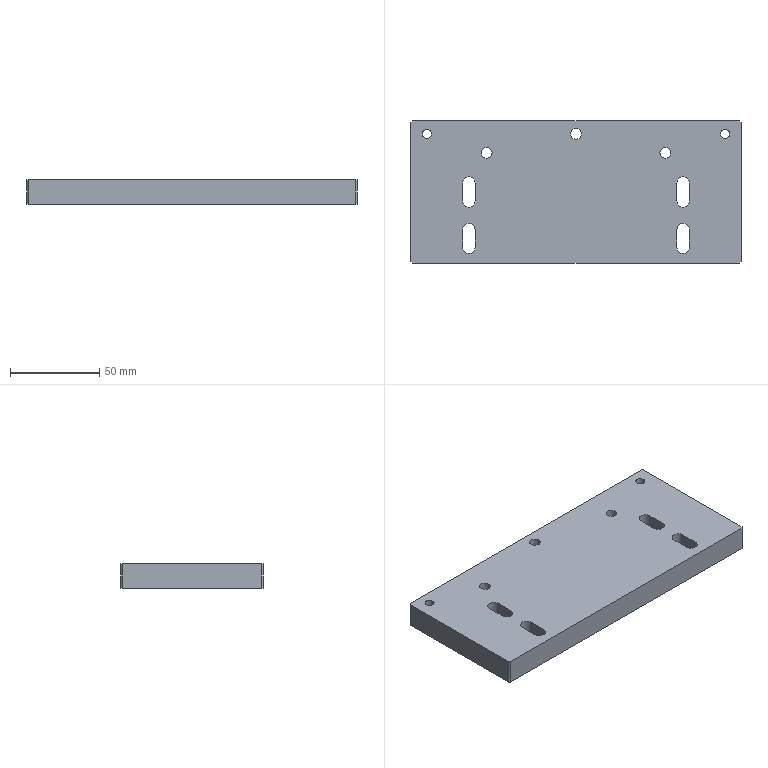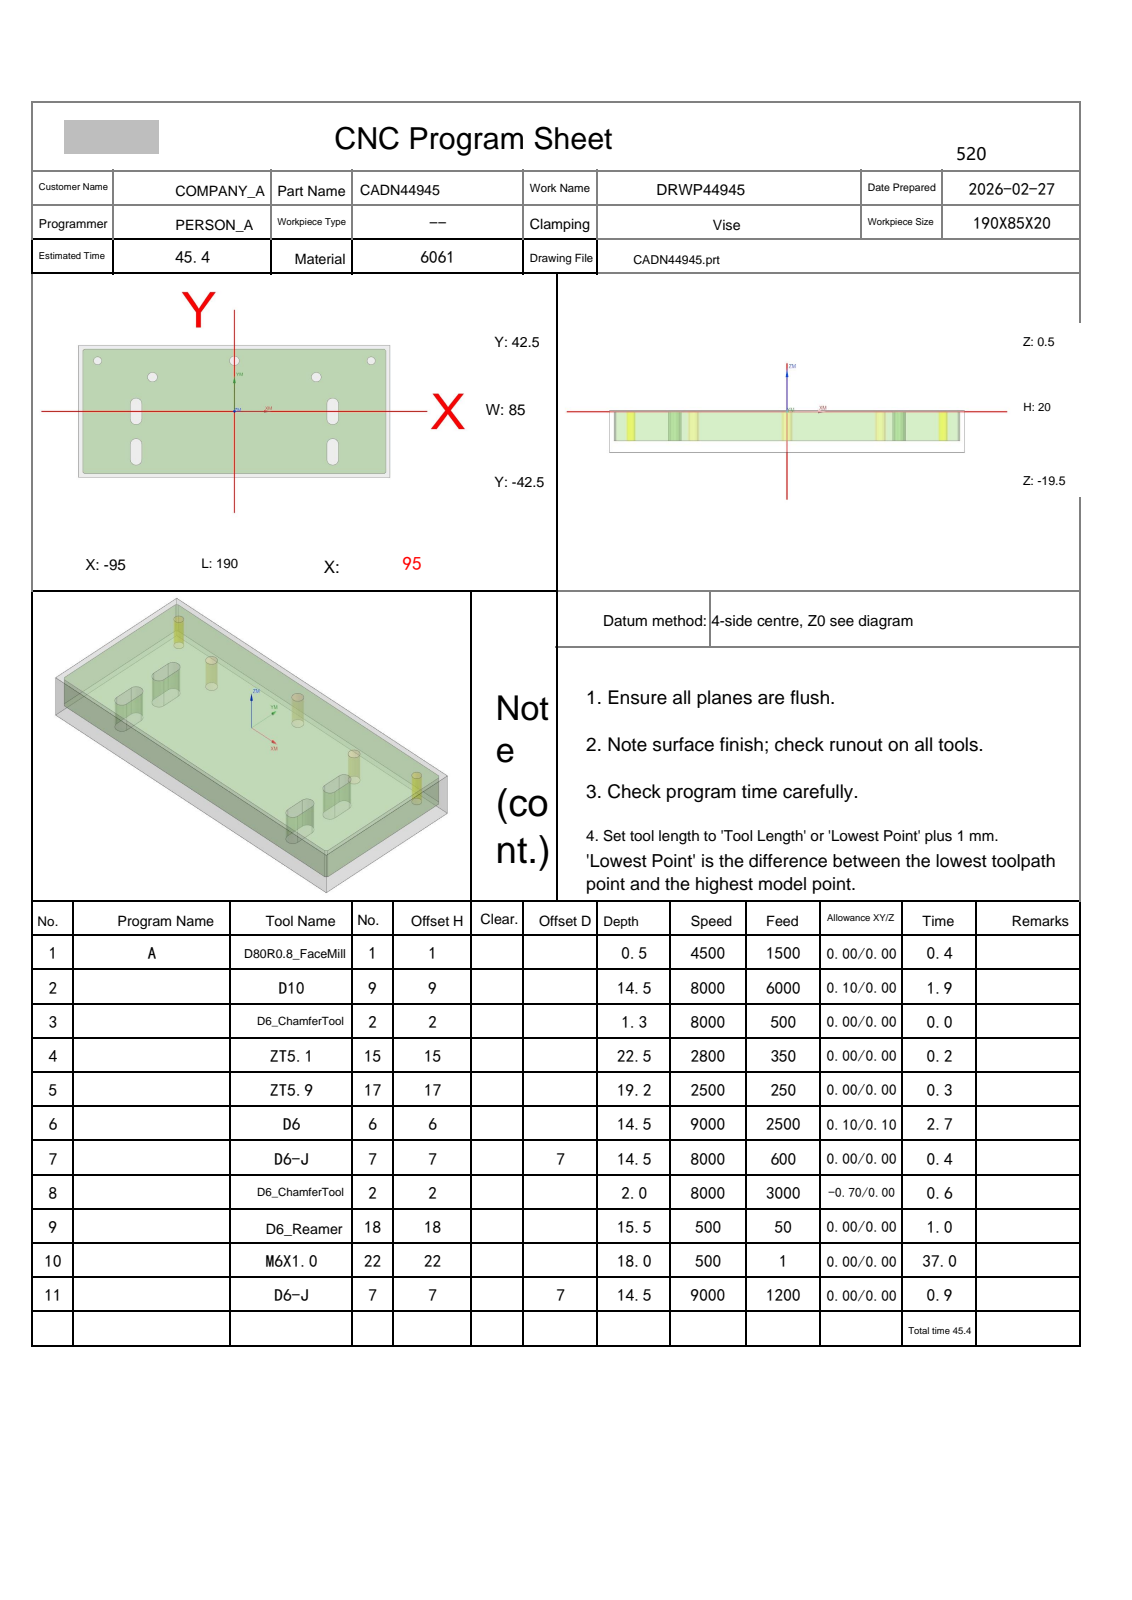NC program | NX | posted by the shop | part box 185 x 80 x 14 mm
Lines 2325 to 2772 of 2772:
N7 T07 M06
(D6-J  D=6. R=0. H=07 ce=0.00 di=0.00)
G00 G90 G54 X-59.75 Y-26.2 M03 S8000
G43 H07 Z50.
M08
Z-6.5
G01 Z-7. F600.
G41 D07
X-59.7
G03 X-59.5 Y-26. I0.0 J.2
G01 Y-21.
G03 X-60. Y-20.5 I-.5 J0.0
X-60.5 Y-21. I0.0 J-.5
G01 Y-31.
G03 X-60. Y-31.5 I.5 J0.0
X-59.5 Y-31. I0.0 J.5
G01 Y-26.
Y-25.5
G03 X-59.7 Y-25.3 I-.2 J0.0
G01 G40 X-59.75
Z-6.5
G00 Z1.
Y-26.2
Z-13.5
G01 Z-14.
G41 D07
X-59.7
G03 X-59.5 Y-26. I0.0 J.2
G01 Y-21.
G03 X-60. Y-20.5 I-.5 J0.0
X-60.5 Y-21. I0.0 J-.5
G01 Y-31.
G03 X-60. Y-31.5 I.5 J0.0
X-59.5 Y-31. I0.0 J.5
G01 Y-26.
Y-25.5
G03 X-59.7 Y-25.3 I-.2 J0.0
G01 G40 X-59.75
Z-13.5
G00 Z50.
Y-.2
Z-6.5
G01 Z-7.
G41 D07
X-59.7
G03 X-59.5 Y0.0 I0.0 J.2
G01 Y5.
G03 X-60. Y5.5 I-.5 J0.0
X-60.5 Y5. I0.0 J-.5
G01 Y-5.
G03 X-60. Y-5.5 I.5 J0.0
X-59.5 Y-5. I0.0 J.5
G01 Y0.0
Y.5
G03 X-59.7 Y.7 I-.2 J0.0
G01 G40 X-59.75
Z-6.5
G00 Z1.
Y-.2
Z-13.5
G01 Z-14.
G41 D07
X-59.7
G03 X-59.5 Y0.0 I0.0 J.2
G01 Y5.
G03 X-60. Y5.5 I-.5 J0.0
X-60.5 Y5. I0.0 J-.5
G01 Y-5.
G03 X-60. Y-5.5 I.5 J0.0
X-59.5 Y-5. I0.0 J.5
G01 Y0.0
Y.5
G03 X-59.7 Y.7 I-.2 J0.0
G01 G40 X-59.75
Z-13.5
G00 Z50.
X60.25 Y-26.2
Z-6.5
G01 Z-7.
G41 D07
X60.3
G03 X60.5 Y-26. I0.0 J.2
G01 Y-21.
G03 X60. Y-20.5 I-.5 J0.0
X59.5 Y-21. I0.0 J-.5
G01 Y-31.
G03 X60. Y-31.5 I.5 J0.0
X60.5 Y-31. I0.0 J.5
G01 Y-26.
Y-25.5
G03 X60.3 Y-25.3 I-.2 J0.0
G01 G40 X60.25
Z-6.5
G00 Z1.
Y-26.2
Z-13.5
G01 Z-14.
G41 D07
X60.3
G03 X60.5 Y-26. I0.0 J.2
G01 Y-21.
G03 X60. Y-20.5 I-.5 J0.0
X59.5 Y-21. I0.0 J-.5
G01 Y-31.
G03 X60. Y-31.5 I.5 J0.0
X60.5 Y-31. I0.0 J.5
G01 Y-26.
Y-25.5
G03 X60.3 Y-25.3 I-.2 J0.0
G01 G40 X60.25
Z-13.5
G00 Z50.
Y-.2
Z-6.5
G01 Z-7.
G41 D07
X60.3
G03 X60.5 Y0.0 I0.0 J.2
G01 Y5.
G03 X60. Y5.5 I-.5 J0.0
X59.5 Y5. I0.0 J-.5
G01 Y-5.
G03 X60. Y-5.5 I.5 J0.0
X60.5 Y-5. I0.0 J.5
G01 Y0.0
Y.5
G03 X60.3 Y.7 I-.2 J0.0
G01 G40 X60.25
Z-6.5
G00 Z1.
Y-.2
Z-13.5
G01 Z-14.
G41 D07
X60.3
G03 X60.5 Y0.0 I0.0 J.2
G01 Y5.
G03 X60. Y5.5 I-.5 J0.0
X59.5 Y5. I0.0 J-.5
G01 Y-5.
G03 X60. Y-5.5 I.5 J0.0
X60.5 Y-5. I0.0 J.5
G01 Y0.0
Y.5
G03 X60.3 Y.7 I-.2 J0.0
G01 G40 X60.25
Z-13.5
G00 Z50.
G91 G28 Z0.0
M05
M09
G91 G28 Z0.0
M01
N8 T02 M06
(D6_ChamferTool  D=6. R=0. H=02 ce=0.00 di=0.00)
G00 G90 G54 X-.25 Y42.128 M03 S8000
G43 H02 Z50.
M08
Z2.099
G01 Z-1.5 F3000.
G03 X-.33 Y41.828 I.52 J-.3
X-.03 Y41.308 I.6 J0.0
G01 X0.0 Y41.3
X91.5
X91.754 Y41.275
X91.997 Y41.201
X92.222 Y41.081
X92.419 Y40.919
X93.419 Y39.919
X93.581 Y39.722
X93.701 Y39.497
X93.775 Y39.254
X93.8 Y39.
Y-39.
X93.775 Y-39.254
X93.701 Y-39.497
X93.581 Y-39.722
X93.419 Y-39.919
X92.419 Y-40.919
X92.222 Y-41.081
X91.997 Y-41.201
X91.754 Y-41.275
X91.5 Y-41.3
X-91.5
X-91.753 Y-41.275
X-91.997 Y-41.201
X-92.222 Y-41.081
X-92.419 Y-40.919
X-93.419 Y-39.919
X-93.581 Y-39.722
X-93.701 Y-39.497
X-93.775 Y-39.254
X-93.8 Y-39.
Y39.
X-93.775 Y39.254
X-93.701 Y39.497
X-93.581 Y39.722
X-93.419 Y39.919
X-92.419 Y40.919
X-92.222 Y41.081
X-91.997 Y41.201
X-91.754 Y41.275
X-91.5 Y41.3
X0.0
X.03 Y41.308
G03 X.33 Y41.828 I-.3 J.52
X.25 Y42.128 I-.6 J0.0
G01 Z2.099
G00 Z50.
X58.628 Y-25.75
Z2.099
G01 Z-1.5
G03 X58.328 Y-25.67 I-.3 J-.52
X57.808 Y-25.97 I0.0 J-.6
G01 X57.8 Y-26.
Y-31.
G03 X60. Y-33.2 I2.2 J0.0
X62.2 Y-31. I0.0 J2.2
G01 Y-21.
G03 X60. Y-18.8 I-2.2 J0.0
X57.8 Y-21. I0.0 J-2.2
G01 Y-26.
X57.808 Y-26.03
G03 X58.328 Y-26.33 I.52 J.3
X58.628 Y-26.25 I0.0 J.6
G01 Z2.099
G00 Z50.
Y.25
Z2.099
G01 Z-1.5
G03 X58.328 Y.33 I-.3 J-.52
X57.808 Y.03 I0.0 J-.6
G01 X57.8 Y0.0
Y-5.
G03 X60. Y-7.2 I2.2 J0.0
X62.2 Y-5. I0.0 J2.2
G01 Y5.
G03 X60. Y7.2 I-2.2 J0.0
X57.8 Y5. I0.0 J-2.2
G01 Y0.0
X57.808 Y-.03
G03 X58.328 Y-.33 I.52 J.3
X58.628 Y-.25 I0.0 J.6
G01 Z2.099
G00 Z50.
X-58.628
Z2.099
G01 Z-1.5
G03 X-58.328 Y-.33 I.3 J.52
X-57.808 Y-.03 I0.0 J.6
G01 X-57.8 Y0.0
Y5.
G03 X-60. Y7.2 I-2.2 J0.0
X-62.2 Y5. I0.0 J-2.2
G01 Y-5.
G03 X-60. Y-7.2 I2.2 J0.0
X-57.8 Y-5. I0.0 J2.2
G01 Y0.0
X-57.808 Y.03
G03 X-58.328 Y.33 I-.52 J-.3
X-58.628 Y.25 I0.0 J-.6
G01 Z2.099
G00 Z50.
Y-26.25
Z2.099
G01 Z-1.5
G03 X-58.328 Y-26.33 I.3 J.52
X-57.808 Y-26.03 I0.0 J.6
G01 X-57.8 Y-26.
Y-21.
G03 X-60. Y-18.8 I-2.2 J0.0
X-62.2 Y-21. I0.0 J-2.2
G01 Y-31.
G03 X-60. Y-33.2 I2.2 J0.0
X-57.8 Y-31. I0.0 J2.2
G01 Y-26.
X-57.808 Y-25.97
G03 X-58.328 Y-25.67 I-.52 J-.3
X-58.628 Y-25.75 I0.0 J-.6
G01 Z2.099
G00 Z50.
G00 G90 X-83.909 Y33.521 M03 S8000
Z50.
Z-.6
G01 Z-1.1 F500.
X-84.1 Y34.
G03 X-85.6 Y32.5 I0.0 J-1.5
X-83.5 Y30.4 I2.1 J0.0
X-81.4 Y32.5 I0.0 J2.1
X-83.5 Y34.6 I-2.1 J0.0
X-85.6 Y32.5 I0.0 J-2.1
X-84.1 Y31. I1.5 J0.0
G01 X-83.909 Y31.479
Z-.6
G00 Z50.
X83.091 Y33.521
Z-.6
G01 Z-1.1
X82.9 Y34.
G03 X81.4 Y32.5 I0.0 J-1.5
X83.5 Y30.4 I2.1 J0.0
X85.6 Y32.5 I0.0 J2.1
X83.5 Y34.6 I-2.1 J0.0
X81.4 Y32.5 I0.0 J-2.1
X82.9 Y31. I1.5 J0.0
G01 X83.091 Y31.479
Z-.6
G00 Z50.
G00 G90 X-50.612 Y23.147 M03 S8000
Z50.
Z-.5
G01 Z-1. F500.
X-50.8 Y23.5
G03 X-52.3 Y22. I0.0 J-1.5
X-50. Y19.7 I2.3 J0.0
X-47.7 Y22. I0.0 J2.3
X-50. Y24.3 I-2.3 J0.0
X-52.3 Y22. I0.0 J-2.3
X-50.8 Y20.5 I1.5 J0.0
G01 X-50.612 Y20.853
Z-.5
G00 Z50.
X-.612 Y33.647
Z-.5
G01 Z-1.
X-.8 Y34.
G03 X-2.3 Y32.5 I0.0 J-1.5
X0.0 Y30.2 I2.3 J0.0
X2.3 Y32.5 I0.0 J2.3
X0.0 Y34.8 I-2.3 J0.0
X-2.3 Y32.5 I0.0 J-2.3
X-.8 Y31. I1.5 J0.0
G01 X-.612 Y31.353
Z-.5
G00 Z50.
X49.388 Y23.147
Z-.5
G01 Z-1.
X49.2 Y23.5
G03 X47.7 Y22. I0.0 J-1.5
X50. Y19.7 I2.3 J0.0
X52.3 Y22. I0.0 J2.3
X50. Y24.3 I-2.3 J0.0
X47.7 Y22. I0.0 J-2.3
X49.2 Y20.5 I1.5 J0.0
G01 X49.388 Y20.853
Z-.5
G00 Z50.
G91 G28 Z0.0
M05
M09
G91 G28 Z0.0
M01
N9 T18 M06
(D6_Reamer D=6. DR_a=180 H=18)
G00 G90 G54 X50. Y22. M03 S500
G43 H18 Z50.
M08
G98 G81 X50. Y22. Z-15. R1. F50.
X0.0 Y32.5
X-50. Y22.
G80
G00 Z50.
G91 G28 Z0.0
M05
M09
G91 G28 Z0.0
M01
N10 T22 M06
(M6X1.0 D=5. DR_a=180 H=22)
G00 G90 G54 X-83.5 Y32.5 M03 S500
G43 H22 Z50.
M08
G95
G98 G84 X-83.5 Y32.5 Z-17.5 R1. F1. Q3.
X83.5
G80
G94
G00 Z50.
G91 G28 Z0.0
M05
M09
G91 G28 Z0.0
M01
N11 T07 M06
(D6-J  D=6. R=0. H=07 ce=0.00 di=0.00)
G00 G90 G54 X92.517 Y-44.073 M03 S9000
G43 H07 Z50.
M08
Z-6.5
G01 Z-7. F1200.
G41 D07
X92.492 Y-43.875
G03 X91.5 Y-43. I-.992 J-.125
G01 X-91.5
G02 X-93.621 Y-42.121 I0.0 J3.
G01 X-94.621 Y-41.121
G02 X-95.5 Y-39. I2.121 J2.121
G01 Y39.
G02 X-94.621 Y41.121 I3. J0.0
G01 X-93.621 Y42.121
G02 X-91.5 Y43. I2.121 J-2.121
G01 X91.5
G02 X93.621 Y42.121 I0.0 J-3.
G01 X94.621 Y41.121
G02 X95.5 Y39. I-2.121 J-2.121
G01 Y-39.
G02 X94.621 Y-41.121 I-3. J0.0
G01 X93.621 Y-42.121
G02 X91.5 Y-43. I-2.121 J2.121
G01 X91.
G03 X90. Y-44. I0.0 J-1.
G01 G40 Y-44.2
Z-6.5
G00 Z50.
X92.517 Y-44.073
Z-13.5
G01 Z-14.
G41 D07
X92.492 Y-43.875
G03 X91.5 Y-43. I-.992 J-.125
G01 X-91.5
G02 X-93.621 Y-42.121 I0.0 J3.
G01 X-94.621 Y-41.121
G02 X-95.5 Y-39. I2.121 J2.121
G01 Y39.
G02 X-94.621 Y41.121 I3. J0.0
G01 X-93.621 Y42.121
G02 X-91.5 Y43. I2.121 J-2.121
G01 X91.5
G02 X93.621 Y42.121 I0.0 J-3.
G01 X94.621 Y41.121
G02 X95.5 Y39. I-2.121 J-2.121
G01 Y-39.
G02 X94.621 Y-41.121 I-3. J0.0
G01 X93.621 Y-42.121
G02 X91.5 Y-43. I-2.121 J2.121
G01 X91.
G03 X90. Y-44. I0.0 J-1.
G01 G40 Y-44.2
Z-13.5
G00 Z50.
M05
M09
G91 G28 Z0.0
G91 G28 Y0.0
M30
%